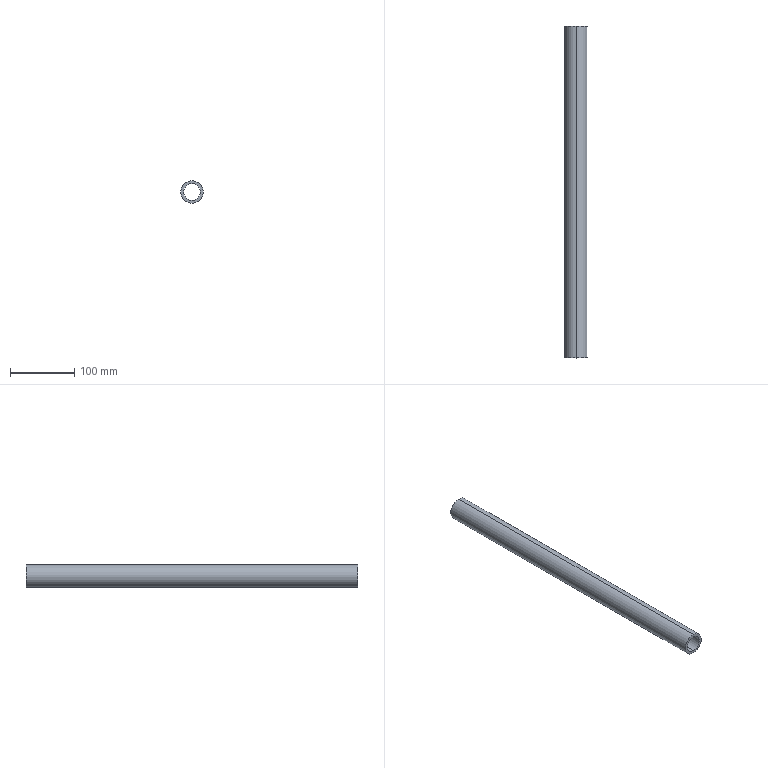Part | SolidWorks | features Extrusion 1, Shell 1 | 1 solid | 6 faces | box 35 x 515 x 35 mm | volume 222060 mm3 | cylinder 4 | plane 2 | commonest cylinder face diameters 26 x2 35 x2
STEP:
#1=CARTESIAN_POINT('',(0.,515.,-13.));
#2=VERTEX_POINT('',#1);
#3=CARTESIAN_POINT('',(0.,515.,13.));
#4=VERTEX_POINT('',#3);
#5=CARTESIAN_POINT('',(0.,515.,0.));
#6=DIRECTION('',(0.,1.,0.));
#7=DIRECTION('',(0.,0.,1.));
#8=AXIS2_PLACEMENT_3D('',#5,#6,#7);
#9=CIRCLE('',#8,13.);
#10=EDGE_CURVE('',#2,#4,#9,.T.);
#11=ORIENTED_EDGE('',*,*,#10,.T.);
#12=CARTESIAN_POINT('',(0.,0.,13.));
#13=VERTEX_POINT('',#12);
#14=CARTESIAN_POINT('',(0.,515.,13.));
#15=DIRECTION('',(0.,-1.,0.));
#16=VECTOR('',#15,1000.);
#17=LINE('',#14,#16);
#18=EDGE_CURVE('',#4,#13,#17,.T.);
#19=ORIENTED_EDGE('',*,*,#18,.T.);
#20=CARTESIAN_POINT('',(0.,0.,-13.));
#21=VERTEX_POINT('',#20);
#22=CARTESIAN_POINT('',(0.,0.,0.));
#23=DIRECTION('',(0.,1.,0.));
#24=DIRECTION('',(0.,0.,1.));
#25=AXIS2_PLACEMENT_3D('',#22,#23,#24);
#26=CIRCLE('',#25,13.);
#27=EDGE_CURVE('',#21,#13,#26,.T.);
#28=ORIENTED_EDGE('',*,*,#27,.F.);
#29=CARTESIAN_POINT('',(0.,515.,-13.));
#30=DIRECTION('',(0.,-1.,0.));
#31=VECTOR('',#30,1000.);
#32=LINE('',#29,#31);
#33=EDGE_CURVE('',#2,#21,#32,.T.);
#34=ORIENTED_EDGE('',*,*,#33,.F.);
#35=EDGE_LOOP('',(#11,#19,#28,#34));
#36=FACE_OUTER_BOUND('',#35,.T.);
#37=CARTESIAN_POINT('',(0.,515.,0.));
#38=DIRECTION('',(0.,-1.,0.));
#39=DIRECTION('',(0.,0.,-1.));
#40=AXIS2_PLACEMENT_3D('',#37,#38,#39);
#41=CYLINDRICAL_SURFACE('',#40,13.);
#42=ADVANCED_FACE('',(#36),#41,.F.);
#43=CARTESIAN_POINT('',(0.,515.,17.5));
#44=VERTEX_POINT('',#43);
#45=CARTESIAN_POINT('',(0.,515.,-17.5));
#46=VERTEX_POINT('',#45);
#47=CARTESIAN_POINT('',(0.,515.,0.));
#48=DIRECTION('',(0.,1.,0.));
#49=DIRECTION('',(0.,0.,1.));
#50=AXIS2_PLACEMENT_3D('',#47,#48,#49);
#51=CIRCLE('',#50,17.5);
#52=EDGE_CURVE('',#44,#46,#51,.T.);
#53=ORIENTED_EDGE('',*,*,#52,.F.);
#54=CARTESIAN_POINT('',(0.,0.,17.5));
#55=VERTEX_POINT('',#54);
#56=CARTESIAN_POINT('',(0.,515.,17.5));
#57=DIRECTION('',(0.,-1.,0.));
#58=VECTOR('',#57,1000.);
#59=LINE('',#56,#58);
#60=EDGE_CURVE('',#44,#55,#59,.T.);
#61=ORIENTED_EDGE('',*,*,#60,.T.);
#62=CARTESIAN_POINT('',(0.,0.,-17.5));
#63=VERTEX_POINT('',#62);
#64=CARTESIAN_POINT('',(0.,0.,0.));
#65=DIRECTION('',(0.,1.,0.));
#66=DIRECTION('',(0.,0.,1.));
#67=AXIS2_PLACEMENT_3D('',#64,#65,#66);
#68=CIRCLE('',#67,17.5);
#69=EDGE_CURVE('',#55,#63,#68,.T.);
#70=ORIENTED_EDGE('',*,*,#69,.T.);
#71=CARTESIAN_POINT('',(0.,515.,-17.5));
#72=DIRECTION('',(0.,-1.,0.));
#73=VECTOR('',#72,1000.);
#74=LINE('',#71,#73);
#75=EDGE_CURVE('',#46,#63,#74,.T.);
#76=ORIENTED_EDGE('',*,*,#75,.F.);
#77=EDGE_LOOP('',(#53,#61,#70,#76));
#78=FACE_OUTER_BOUND('',#77,.T.);
#79=CARTESIAN_POINT('',(0.,515.,0.));
#80=DIRECTION('',(0.,-1.,0.));
#81=DIRECTION('',(0.,0.,-1.));
#82=AXIS2_PLACEMENT_3D('',#79,#80,#81);
#83=CYLINDRICAL_SURFACE('',#82,17.5);
#84=ADVANCED_FACE('',(#78),#83,.T.);
#85=ORIENTED_EDGE('',*,*,#60,.F.);
#86=CARTESIAN_POINT('',(0.,515.,0.));
#87=DIRECTION('',(0.,1.,0.));
#88=DIRECTION('',(0.,0.,1.));
#89=AXIS2_PLACEMENT_3D('',#86,#87,#88);
#90=CIRCLE('',#89,17.5);
#91=EDGE_CURVE('',#46,#44,#90,.T.);
#92=ORIENTED_EDGE('',*,*,#91,.F.);
#93=ORIENTED_EDGE('',*,*,#75,.T.);
#94=CARTESIAN_POINT('',(0.,0.,0.));
#95=DIRECTION('',(0.,1.,0.));
#96=DIRECTION('',(0.,0.,1.));
#97=AXIS2_PLACEMENT_3D('',#94,#95,#96);
#98=CIRCLE('',#97,17.5);
#99=EDGE_CURVE('',#63,#55,#98,.T.);
#100=ORIENTED_EDGE('',*,*,#99,.T.);
#101=EDGE_LOOP('',(#85,#92,#93,#100));
#102=FACE_OUTER_BOUND('',#101,.T.);
#103=CARTESIAN_POINT('',(0.,515.,0.));
#104=DIRECTION('',(0.,-1.,0.));
#105=DIRECTION('',(0.,0.,-1.));
#106=AXIS2_PLACEMENT_3D('',#103,#104,#105);
#107=CYLINDRICAL_SURFACE('',#106,17.5);
#108=ADVANCED_FACE('',(#102),#107,.T.);
#109=ORIENTED_EDGE('',*,*,#10,.F.);
#110=CARTESIAN_POINT('',(0.,515.,0.));
#111=DIRECTION('',(0.,1.,0.));
#112=DIRECTION('',(0.,0.,1.));
#113=AXIS2_PLACEMENT_3D('',#110,#111,#112);
#114=CIRCLE('',#113,13.);
#115=EDGE_CURVE('',#4,#2,#114,.T.);
#116=ORIENTED_EDGE('',*,*,#115,.F.);
#117=EDGE_LOOP('',(#109,#116));
#118=FACE_BOUND('',#117,.T.);
#119=ORIENTED_EDGE('',*,*,#91,.T.);
#120=ORIENTED_EDGE('',*,*,#52,.T.);
#121=EDGE_LOOP('',(#119,#120));
#122=FACE_OUTER_BOUND('',#121,.T.);
#123=CARTESIAN_POINT('',(0.,515.,0.));
#124=DIRECTION('',(0.,1.,0.));
#125=DIRECTION('',(0.,0.,1.));
#126=AXIS2_PLACEMENT_3D('',#123,#124,#125);
#127=PLANE('',#126);
#128=ADVANCED_FACE('',(#118,#122),#127,.T.);
#129=ORIENTED_EDGE('',*,*,#27,.T.);
#130=CARTESIAN_POINT('',(0.,0.,0.));
#131=DIRECTION('',(0.,1.,0.));
#132=DIRECTION('',(0.,0.,1.));
#133=AXIS2_PLACEMENT_3D('',#130,#131,#132);
#134=CIRCLE('',#133,13.);
#135=EDGE_CURVE('',#13,#21,#134,.T.);
#136=ORIENTED_EDGE('',*,*,#135,.T.);
#137=EDGE_LOOP('',(#129,#136));
#138=FACE_BOUND('',#137,.T.);
#139=ORIENTED_EDGE('',*,*,#99,.F.);
#140=ORIENTED_EDGE('',*,*,#69,.F.);
#141=EDGE_LOOP('',(#139,#140));
#142=FACE_OUTER_BOUND('',#141,.T.);
#143=CARTESIAN_POINT('',(0.,0.,0.));
#144=DIRECTION('',(0.,1.,0.));
#145=DIRECTION('',(0.,0.,1.));
#146=AXIS2_PLACEMENT_3D('',#143,#144,#145);
#147=PLANE('',#146);
#148=ADVANCED_FACE('',(#138,#142),#147,.F.);
#149=ORIENTED_EDGE('',*,*,#18,.F.);
#150=ORIENTED_EDGE('',*,*,#115,.T.);
#151=ORIENTED_EDGE('',*,*,#33,.T.);
#152=ORIENTED_EDGE('',*,*,#135,.F.);
#153=EDGE_LOOP('',(#149,#150,#151,#152));
#154=FACE_OUTER_BOUND('',#153,.T.);
#155=CARTESIAN_POINT('',(0.,515.,0.));
#156=DIRECTION('',(0.,-1.,0.));
#157=DIRECTION('',(0.,0.,-1.));
#158=AXIS2_PLACEMENT_3D('',#155,#156,#157);
#159=CYLINDRICAL_SURFACE('',#158,13.);
#160=ADVANCED_FACE('',(#154),#159,.F.);
#161=CLOSED_SHELL('',(#42,#84,#108,#128,#148,#160));
#162=MANIFOLD_SOLID_BREP('',#161);
#163=CARTESIAN_POINT('',(0.,0.,0.));
#164=DIRECTION('',(0.,0.,1.));
#165=DIRECTION('',(1.,0.,0.));
#166=AXIS2_PLACEMENT_3D('',#163,#164,#165);
#167=(LENGTH_UNIT()NAMED_UNIT(*)SI_UNIT(.MILLI.,.METRE.));
#168=UNCERTAINTY_MEASURE_WITH_UNIT(LENGTH_MEASURE(0.00001),#167,'','');
#169=(NAMED_UNIT(*)PLANE_ANGLE_UNIT()SI_UNIT($,.RADIAN.));
#170=(NAMED_UNIT(*)SI_UNIT($,.STERADIAN.)SOLID_ANGLE_UNIT());
#171=(GEOMETRIC_REPRESENTATION_CONTEXT(3)GLOBAL_UNCERTAINTY_ASSIGNED_CONTEXT((#168))GLOBAL_UNIT_ASSIGNED_CONTEXT((#167,#169,#170))REPRESENTATION_CONTEXT('',''));
#172=ADVANCED_BREP_SHAPE_REPRESENTATION('',(#162,#166),#171);